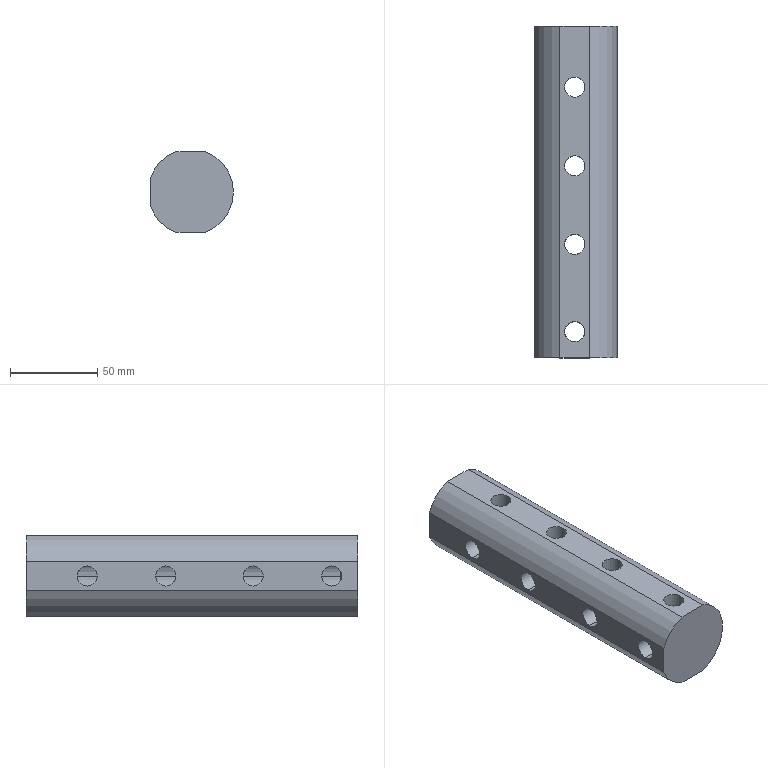Part | SolidWorks | features BaseBody 1 | 1 solid | 36 faces | box 47.5 x 190 x 46 mm | volume 274683 mm3 | cylinder 29 | plane 5 | cone 2 | commonest cylinder face diameters 11.5 x24 49 x3 20 x2